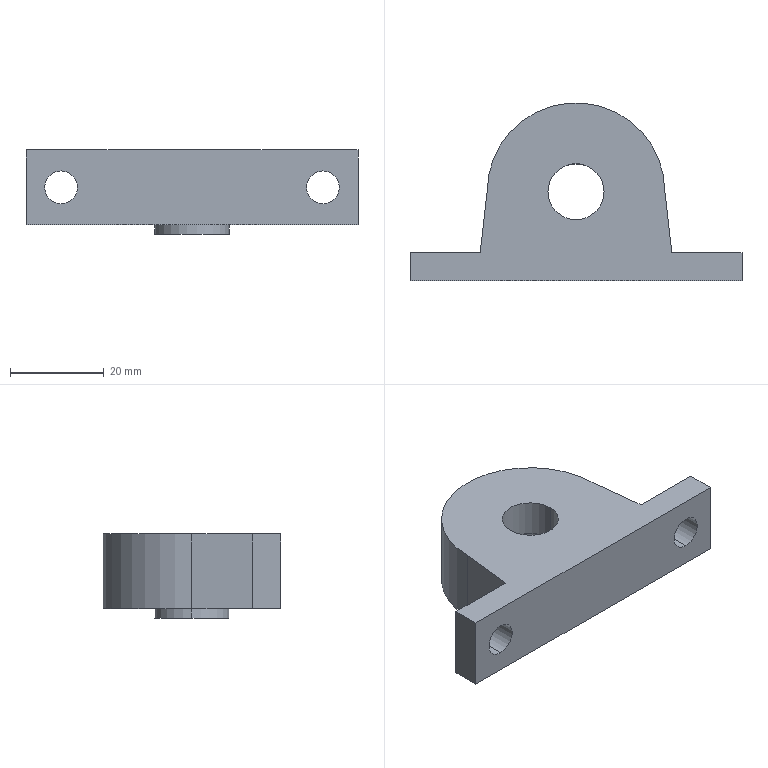Part | 2 solids | 22 faces | box 71 x 38 x 18 mm | volume 22713 mm3 | cylinder 11 | plane 11 | commonest cylinder face diameters 7 x4 12 x4 16 x2 38 x1
STEP:
#1=CARTESIAN_POINT('',(28.,-19.,4.5));
#2=VERTEX_POINT('',#1);
#3=CARTESIAN_POINT('',(28.,-19.,11.5));
#4=VERTEX_POINT('',#3);
#5=CARTESIAN_POINT('',(28.,-19.,8.));
#6=DIRECTION('',(0.,1.,0.));
#7=DIRECTION('',(-1.,0.,0.));
#8=AXIS2_PLACEMENT_3D('',#5,#6,#7);
#9=CIRCLE('',#8,3.5);
#10=EDGE_CURVE('',#2,#4,#9,.T.);
#11=ORIENTED_EDGE('',*,*,#10,.F.);
#12=CARTESIAN_POINT('',(28.,-13.,4.5));
#13=VERTEX_POINT('',#12);
#14=CARTESIAN_POINT('',(28.,-23.,4.5));
#15=DIRECTION('',(0.,1.,0.));
#16=VECTOR('',#15,1000.);
#17=LINE('',#14,#16);
#18=EDGE_CURVE('',#2,#13,#17,.T.);
#19=ORIENTED_EDGE('',*,*,#18,.T.);
#20=CARTESIAN_POINT('',(28.,-13.,11.5));
#21=VERTEX_POINT('',#20);
#22=CARTESIAN_POINT('',(28.,-13.,8.));
#23=DIRECTION('',(0.,1.,0.));
#24=DIRECTION('',(0.,0.,1.));
#25=AXIS2_PLACEMENT_3D('',#22,#23,#24);
#26=CIRCLE('',#25,3.5);
#27=EDGE_CURVE('',#13,#21,#26,.T.);
#28=ORIENTED_EDGE('',*,*,#27,.T.);
#29=CARTESIAN_POINT('',(28.,-23.,11.5));
#30=DIRECTION('',(0.,1.,0.));
#31=VECTOR('',#30,1000.);
#32=LINE('',#29,#31);
#33=EDGE_CURVE('',#4,#21,#32,.T.);
#34=ORIENTED_EDGE('',*,*,#33,.F.);
#35=EDGE_LOOP('',(#11,#19,#28,#34));
#36=FACE_OUTER_BOUND('',#35,.T.);
#37=CARTESIAN_POINT('',(28.,-23.,8.));
#38=DIRECTION('',(0.,1.,0.));
#39=DIRECTION('',(0.,0.,1.));
#40=AXIS2_PLACEMENT_3D('',#37,#38,#39);
#41=CYLINDRICAL_SURFACE('',#40,3.5);
#42=ADVANCED_FACE('',(#36),#41,.F.);
#43=CARTESIAN_POINT('',(-28.,-19.,4.5));
#44=VERTEX_POINT('',#43);
#45=CARTESIAN_POINT('',(-28.,-19.,11.5));
#46=VERTEX_POINT('',#45);
#47=CARTESIAN_POINT('',(-28.,-19.,8.));
#48=DIRECTION('',(0.,1.,0.));
#49=DIRECTION('',(-1.,0.,0.));
#50=AXIS2_PLACEMENT_3D('',#47,#48,#49);
#51=CIRCLE('',#50,3.5);
#52=EDGE_CURVE('',#44,#46,#51,.T.);
#53=ORIENTED_EDGE('',*,*,#52,.F.);
#54=CARTESIAN_POINT('',(-28.,-13.,4.5));
#55=VERTEX_POINT('',#54);
#56=CARTESIAN_POINT('',(-28.,-23.,4.5));
#57=DIRECTION('',(0.,1.,0.));
#58=VECTOR('',#57,1000.);
#59=LINE('',#56,#58);
#60=EDGE_CURVE('',#44,#55,#59,.T.);
#61=ORIENTED_EDGE('',*,*,#60,.T.);
#62=CARTESIAN_POINT('',(-28.,-13.,11.5));
#63=VERTEX_POINT('',#62);
#64=CARTESIAN_POINT('',(-28.,-13.,8.));
#65=DIRECTION('',(0.,1.,0.));
#66=DIRECTION('',(0.,0.,1.));
#67=AXIS2_PLACEMENT_3D('',#64,#65,#66);
#68=CIRCLE('',#67,3.5);
#69=EDGE_CURVE('',#55,#63,#68,.T.);
#70=ORIENTED_EDGE('',*,*,#69,.T.);
#71=CARTESIAN_POINT('',(-28.,-23.,11.5));
#72=DIRECTION('',(0.,1.,0.));
#73=VECTOR('',#72,1000.);
#74=LINE('',#71,#73);
#75=EDGE_CURVE('',#46,#63,#74,.T.);
#76=ORIENTED_EDGE('',*,*,#75,.F.);
#77=EDGE_LOOP('',(#53,#61,#70,#76));
#78=FACE_OUTER_BOUND('',#77,.T.);
#79=CARTESIAN_POINT('',(-28.,-23.,8.));
#80=DIRECTION('',(0.,1.,0.));
#81=DIRECTION('',(0.,0.,1.));
#82=AXIS2_PLACEMENT_3D('',#79,#80,#81);
#83=CYLINDRICAL_SURFACE('',#82,3.5);
#84=ADVANCED_FACE('',(#78),#83,.F.);
#85=CARTESIAN_POINT('',(-6.,0.,16.));
#86=VERTEX_POINT('',#85);
#87=CARTESIAN_POINT('',(6.,0.,16.));
#88=VERTEX_POINT('',#87);
#89=CARTESIAN_POINT('',(0.,0.,16.));
#90=DIRECTION('',(0.,0.,1.));
#91=DIRECTION('',(1.,0.,0.));
#92=AXIS2_PLACEMENT_3D('',#89,#90,#91);
#93=CIRCLE('',#92,6.);
#94=EDGE_CURVE('',#86,#88,#93,.T.);
#95=ORIENTED_EDGE('',*,*,#94,.T.);
#96=CARTESIAN_POINT('',(6.,0.,0.));
#97=VERTEX_POINT('',#96);
#98=CARTESIAN_POINT('',(6.,0.,16.));
#99=DIRECTION('',(0.,0.,-1.));
#100=VECTOR('',#99,1000.);
#101=LINE('',#98,#100);
#102=EDGE_CURVE('',#88,#97,#101,.T.);
#103=ORIENTED_EDGE('',*,*,#102,.T.);
#104=CARTESIAN_POINT('',(-6.,0.,0.));
#105=VERTEX_POINT('',#104);
#106=CARTESIAN_POINT('',(0.,0.,0.));
#107=DIRECTION('',(0.,0.,1.));
#108=DIRECTION('',(1.,0.,0.));
#109=AXIS2_PLACEMENT_3D('',#106,#107,#108);
#110=CIRCLE('',#109,6.);
#111=EDGE_CURVE('',#105,#97,#110,.T.);
#112=ORIENTED_EDGE('',*,*,#111,.F.);
#113=CARTESIAN_POINT('',(-6.,0.,16.));
#114=DIRECTION('',(0.,0.,-1.));
#115=VECTOR('',#114,1000.);
#116=LINE('',#113,#115);
#117=EDGE_CURVE('',#86,#105,#116,.T.);
#118=ORIENTED_EDGE('',*,*,#117,.F.);
#119=EDGE_LOOP('',(#95,#103,#112,#118));
#120=FACE_OUTER_BOUND('',#119,.T.);
#121=CARTESIAN_POINT('',(0.,0.,16.));
#122=DIRECTION('',(0.,0.,-1.));
#123=DIRECTION('',(-1.,0.,0.));
#124=AXIS2_PLACEMENT_3D('',#121,#122,#123);
#125=CYLINDRICAL_SURFACE('',#124,6.);
#126=ADVANCED_FACE('',(#120),#125,.F.);
#127=CARTESIAN_POINT('',(35.5,-13.,16.));
#128=VERTEX_POINT('',#127);
#129=CARTESIAN_POINT('',(20.5,-13.,16.));
#130=VERTEX_POINT('',#129);
#131=CARTESIAN_POINT('',(35.5,-13.,16.));
#132=DIRECTION('',(-1.,0.,0.));
#133=VECTOR('',#132,1000.);
#134=LINE('',#131,#133);
#135=EDGE_CURVE('',#128,#130,#134,.T.);
#136=ORIENTED_EDGE('',*,*,#135,.T.);
#137=CARTESIAN_POINT('',(19.,0.,16.));
#138=VERTEX_POINT('',#137);
#139=CARTESIAN_POINT('',(20.5,-13.,16.));
#140=DIRECTION('',(-0.1146,0.9934,0.));
#141=VECTOR('',#140,1000.);
#142=LINE('',#139,#141);
#143=EDGE_CURVE('',#130,#138,#142,.T.);
#144=ORIENTED_EDGE('',*,*,#143,.T.);
#145=CARTESIAN_POINT('',(-19.,0.,16.));
#146=VERTEX_POINT('',#145);
#147=CARTESIAN_POINT('',(0.,0.,16.));
#148=DIRECTION('',(0.,0.,1.));
#149=DIRECTION('',(1.,0.,0.));
#150=AXIS2_PLACEMENT_3D('',#147,#148,#149);
#151=CIRCLE('',#150,19.);
#152=EDGE_CURVE('',#138,#146,#151,.T.);
#153=ORIENTED_EDGE('',*,*,#152,.T.);
#154=CARTESIAN_POINT('',(-20.5,-13.,16.));
#155=VERTEX_POINT('',#154);
#156=CARTESIAN_POINT('',(-20.5,-13.,16.));
#157=DIRECTION('',(-0.1146,-0.9934,0.));
#158=VECTOR('',#157,1000.);
#159=LINE('',#156,#158);
#160=EDGE_CURVE('',#146,#155,#159,.T.);
#161=ORIENTED_EDGE('',*,*,#160,.T.);
#162=CARTESIAN_POINT('',(-35.5,-13.,16.));
#163=VERTEX_POINT('',#162);
#164=CARTESIAN_POINT('',(-35.5,-13.,16.));
#165=DIRECTION('',(-1.,0.,0.));
#166=VECTOR('',#165,1000.);
#167=LINE('',#164,#166);
#168=EDGE_CURVE('',#155,#163,#167,.T.);
#169=ORIENTED_EDGE('',*,*,#168,.T.);
#170=CARTESIAN_POINT('',(-35.5,-19.,16.));
#171=VERTEX_POINT('',#170);
#172=CARTESIAN_POINT('',(-35.5,-13.,16.));
#173=DIRECTION('',(0.,-1.,0.));
#174=VECTOR('',#173,1000.);
#175=LINE('',#172,#174);
#176=EDGE_CURVE('',#163,#171,#175,.T.);
#177=ORIENTED_EDGE('',*,*,#176,.T.);
#178=CARTESIAN_POINT('',(35.5,-19.,16.));
#179=VERTEX_POINT('',#178);
#180=CARTESIAN_POINT('',(-35.5,-19.,16.));
#181=DIRECTION('',(1.,0.,0.));
#182=VECTOR('',#181,1000.);
#183=LINE('',#180,#182);
#184=EDGE_CURVE('',#171,#179,#183,.T.);
#185=ORIENTED_EDGE('',*,*,#184,.T.);
#186=CARTESIAN_POINT('',(35.5,-19.,16.));
#187=DIRECTION('',(0.,1.,0.));
#188=VECTOR('',#187,1000.);
#189=LINE('',#186,#188);
#190=EDGE_CURVE('',#179,#128,#189,.T.);
#191=ORIENTED_EDGE('',*,*,#190,.T.);
#192=EDGE_LOOP('',(#136,#144,#153,#161,#169,#177,#185,#191));
#193=FACE_OUTER_BOUND('',#192,.T.);
#194=ORIENTED_EDGE('',*,*,#94,.F.);
#195=CARTESIAN_POINT('',(0.,0.,16.));
#196=DIRECTION('',(0.,0.,1.));
#197=DIRECTION('',(1.,0.,0.));
#198=AXIS2_PLACEMENT_3D('',#195,#196,#197);
#199=CIRCLE('',#198,6.);
#200=EDGE_CURVE('',#88,#86,#199,.T.);
#201=ORIENTED_EDGE('',*,*,#200,.F.);
#202=EDGE_LOOP('',(#194,#201));
#203=FACE_BOUND('',#202,.T.);
#204=CARTESIAN_POINT('',(0.,0.,16.));
#205=DIRECTION('',(0.,0.,1.));
#206=DIRECTION('',(1.,0.,0.));
#207=AXIS2_PLACEMENT_3D('',#204,#205,#206);
#208=PLANE('',#207);
#209=ADVANCED_FACE('',(#193,#203),#208,.T.);
#210=CARTESIAN_POINT('',(35.5,-13.,0.));
#211=VERTEX_POINT('',#210);
#212=CARTESIAN_POINT('',(20.5,-13.,0.));
#213=VERTEX_POINT('',#212);
#214=CARTESIAN_POINT('',(35.5,-13.,0.));
#215=DIRECTION('',(-1.,0.,0.));
#216=VECTOR('',#215,1000.);
#217=LINE('',#214,#216);
#218=EDGE_CURVE('',#211,#213,#217,.T.);
#219=ORIENTED_EDGE('',*,*,#218,.F.);
#220=CARTESIAN_POINT('',(35.5,-19.,0.));
#221=VERTEX_POINT('',#220);
#222=CARTESIAN_POINT('',(35.5,-19.,0.));
#223=DIRECTION('',(0.,1.,0.));
#224=VECTOR('',#223,1000.);
#225=LINE('',#222,#224);
#226=EDGE_CURVE('',#221,#211,#225,.T.);
#227=ORIENTED_EDGE('',*,*,#226,.F.);
#228=CARTESIAN_POINT('',(-35.5,-19.,0.));
#229=VERTEX_POINT('',#228);
#230=CARTESIAN_POINT('',(-35.5,-19.,0.));
#231=DIRECTION('',(1.,0.,0.));
#232=VECTOR('',#231,1000.);
#233=LINE('',#230,#232);
#234=EDGE_CURVE('',#229,#221,#233,.T.);
#235=ORIENTED_EDGE('',*,*,#234,.F.);
#236=CARTESIAN_POINT('',(-35.5,-13.,0.));
#237=VERTEX_POINT('',#236);
#238=CARTESIAN_POINT('',(-35.5,-13.,0.));
#239=DIRECTION('',(0.,-1.,0.));
#240=VECTOR('',#239,1000.);
#241=LINE('',#238,#240);
#242=EDGE_CURVE('',#237,#229,#241,.T.);
#243=ORIENTED_EDGE('',*,*,#242,.F.);
#244=CARTESIAN_POINT('',(-20.5,-13.,0.));
#245=VERTEX_POINT('',#244);
#246=CARTESIAN_POINT('',(-35.5,-13.,0.));
#247=DIRECTION('',(-1.,0.,0.));
#248=VECTOR('',#247,1000.);
#249=LINE('',#246,#248);
#250=EDGE_CURVE('',#245,#237,#249,.T.);
#251=ORIENTED_EDGE('',*,*,#250,.F.);
#252=CARTESIAN_POINT('',(-19.,0.,0.));
#253=VERTEX_POINT('',#252);
#254=CARTESIAN_POINT('',(-20.5,-13.,0.));
#255=DIRECTION('',(-0.1146,-0.9934,0.));
#256=VECTOR('',#255,1000.);
#257=LINE('',#254,#256);
#258=EDGE_CURVE('',#253,#245,#257,.T.);
#259=ORIENTED_EDGE('',*,*,#258,.F.);
#260=CARTESIAN_POINT('',(19.,0.,0.));
#261=VERTEX_POINT('',#260);
#262=CARTESIAN_POINT('',(0.,0.,0.));
#263=DIRECTION('',(0.,0.,1.));
#264=DIRECTION('',(1.,0.,0.));
#265=AXIS2_PLACEMENT_3D('',#262,#263,#264);
#266=CIRCLE('',#265,19.);
#267=EDGE_CURVE('',#261,#253,#266,.T.);
#268=ORIENTED_EDGE('',*,*,#267,.F.);
#269=CARTESIAN_POINT('',(20.5,-13.,0.));
#270=DIRECTION('',(-0.1146,0.9934,0.));
#271=VECTOR('',#270,1000.);
#272=LINE('',#269,#271);
#273=EDGE_CURVE('',#213,#261,#272,.T.);
#274=ORIENTED_EDGE('',*,*,#273,.F.);
#275=EDGE_LOOP('',(#219,#227,#235,#243,#251,#259,#268,#274));
#276=FACE_OUTER_BOUND('',#275,.T.);
#277=ORIENTED_EDGE('',*,*,#111,.T.);
#278=CARTESIAN_POINT('',(0.,0.,0.));
#279=DIRECTION('',(0.,0.,1.));
#280=DIRECTION('',(1.,0.,0.));
#281=AXIS2_PLACEMENT_3D('',#278,#279,#280);
#282=CIRCLE('',#281,6.);
#283=EDGE_CURVE('',#97,#105,#282,.T.);
#284=ORIENTED_EDGE('',*,*,#283,.T.);
#285=EDGE_LOOP('',(#277,#284));
#286=FACE_BOUND('',#285,.T.);
#287=CARTESIAN_POINT('',(0.,0.,0.));
#288=DIRECTION('',(0.,0.,1.));
#289=DIRECTION('',(1.,0.,0.));
#290=AXIS2_PLACEMENT_3D('',#287,#288,#289);
#291=PLANE('',#290);
#292=ADVANCED_FACE('',(#276,#286),#291,.F.);
#293=CARTESIAN_POINT('',(28.,-13.,8.));
#294=DIRECTION('',(0.,1.,0.));
#295=DIRECTION('',(0.,0.,1.));
#296=AXIS2_PLACEMENT_3D('',#293,#294,#295);
#297=CIRCLE('',#296,3.5);
#298=EDGE_CURVE('',#21,#13,#297,.T.);
#299=ORIENTED_EDGE('',*,*,#298,.F.);
#300=ORIENTED_EDGE('',*,*,#27,.F.);
#301=EDGE_LOOP('',(#299,#300));
#302=FACE_BOUND('',#301,.T.);
#303=ORIENTED_EDGE('',*,*,#218,.T.);
#304=CARTESIAN_POINT('',(20.5,-13.,16.));
#305=DIRECTION('',(0.,0.,-1.));
#306=VECTOR('',#305,1000.);
#307=LINE('',#304,#306);
#308=EDGE_CURVE('',#130,#213,#307,.T.);
#309=ORIENTED_EDGE('',*,*,#308,.F.);
#310=ORIENTED_EDGE('',*,*,#135,.F.);
#311=CARTESIAN_POINT('',(35.5,-13.,16.));
#312=DIRECTION('',(0.,0.,-1.));
#313=VECTOR('',#312,1000.);
#314=LINE('',#311,#313);
#315=EDGE_CURVE('',#128,#211,#314,.T.);
#316=ORIENTED_EDGE('',*,*,#315,.T.);
#317=EDGE_LOOP('',(#303,#309,#310,#316));
#318=FACE_OUTER_BOUND('',#317,.T.);
#319=CARTESIAN_POINT('',(35.5,-13.,16.));
#320=DIRECTION('',(0.,-1.,0.));
#321=DIRECTION('',(1.,0.,0.));
#322=AXIS2_PLACEMENT_3D('',#319,#320,#321);
#323=PLANE('',#322);
#324=ADVANCED_FACE('',(#302,#318),#323,.F.);
#325=ORIENTED_EDGE('',*,*,#273,.T.);
#326=CARTESIAN_POINT('',(19.,0.,16.));
#327=DIRECTION('',(0.,0.,-1.));
#328=VECTOR('',#327,1000.);
#329=LINE('',#326,#328);
#330=EDGE_CURVE('',#138,#261,#329,.T.);
#331=ORIENTED_EDGE('',*,*,#330,.F.);
#332=ORIENTED_EDGE('',*,*,#143,.F.);
#333=ORIENTED_EDGE('',*,*,#308,.T.);
#334=EDGE_LOOP('',(#325,#331,#332,#333));
#335=FACE_OUTER_BOUND('',#334,.T.);
#336=CARTESIAN_POINT('',(20.5,-13.,16.));
#337=DIRECTION('',(-0.9934,-0.1146,0.));
#338=DIRECTION('',(0.1146,-0.9934,0.));
#339=AXIS2_PLACEMENT_3D('',#336,#337,#338);
#340=PLANE('',#339);
#341=ADVANCED_FACE('',(#335),#340,.F.);
#342=ORIENTED_EDGE('',*,*,#267,.T.);
#343=CARTESIAN_POINT('',(-19.,0.,16.));
#344=DIRECTION('',(0.,0.,-1.));
#345=VECTOR('',#344,1000.);
#346=LINE('',#343,#345);
#347=EDGE_CURVE('',#146,#253,#346,.T.);
#348=ORIENTED_EDGE('',*,*,#347,.F.);
#349=ORIENTED_EDGE('',*,*,#152,.F.);
#350=ORIENTED_EDGE('',*,*,#330,.T.);
#351=EDGE_LOOP('',(#342,#348,#349,#350));
#352=FACE_OUTER_BOUND('',#351,.T.);
#353=CARTESIAN_POINT('',(0.,0.,16.));
#354=DIRECTION('',(0.,0.,-1.));
#355=DIRECTION('',(-1.,0.,0.));
#356=AXIS2_PLACEMENT_3D('',#353,#354,#355);
#357=CYLINDRICAL_SURFACE('',#356,19.);
#358=ADVANCED_FACE('',(#352),#357,.T.);
#359=ORIENTED_EDGE('',*,*,#258,.T.);
#360=CARTESIAN_POINT('',(-20.5,-13.,16.));
#361=DIRECTION('',(0.,0.,-1.));
#362=VECTOR('',#361,1000.);
#363=LINE('',#360,#362);
#364=EDGE_CURVE('',#155,#245,#363,.T.);
#365=ORIENTED_EDGE('',*,*,#364,.F.);
#366=ORIENTED_EDGE('',*,*,#160,.F.);
#367=ORIENTED_EDGE('',*,*,#347,.T.);
#368=EDGE_LOOP('',(#359,#365,#366,#367));
#369=FACE_OUTER_BOUND('',#368,.T.);
#370=CARTESIAN_POINT('',(-20.5,-13.,16.));
#371=DIRECTION('',(0.9934,-0.1146,0.));
#372=DIRECTION('',(0.1146,0.9934,0.));
#373=AXIS2_PLACEMENT_3D('',#370,#371,#372);
#374=PLANE('',#373);
#375=ADVANCED_FACE('',(#369),#374,.F.);
#376=CARTESIAN_POINT('',(-28.,-13.,8.));
#377=DIRECTION('',(0.,1.,0.));
#378=DIRECTION('',(0.,0.,1.));
#379=AXIS2_PLACEMENT_3D('',#376,#377,#378);
#380=CIRCLE('',#379,3.5);
#381=EDGE_CURVE('',#63,#55,#380,.T.);
#382=ORIENTED_EDGE('',*,*,#381,.F.);
#383=ORIENTED_EDGE('',*,*,#69,.F.);
#384=EDGE_LOOP('',(#382,#383));
#385=FACE_BOUND('',#384,.T.);
#386=ORIENTED_EDGE('',*,*,#250,.T.);
#387=CARTESIAN_POINT('',(-35.5,-13.,16.));
#388=DIRECTION('',(0.,0.,-1.));
#389=VECTOR('',#388,1000.);
#390=LINE('',#387,#389);
#391=EDGE_CURVE('',#163,#237,#390,.T.);
#392=ORIENTED_EDGE('',*,*,#391,.F.);
#393=ORIENTED_EDGE('',*,*,#168,.F.);
#394=ORIENTED_EDGE('',*,*,#364,.T.);
#395=EDGE_LOOP('',(#386,#392,#393,#394));
#396=FACE_OUTER_BOUND('',#395,.T.);
#397=CARTESIAN_POINT('',(-35.5,-13.,16.));
#398=DIRECTION('',(0.,-1.,0.));
#399=DIRECTION('',(0.,0.,-1.));
#400=AXIS2_PLACEMENT_3D('',#397,#398,#399);
#401=PLANE('',#400);
#402=ADVANCED_FACE('',(#385,#396),#401,.F.);
#403=ORIENTED_EDGE('',*,*,#242,.T.);
#404=CARTESIAN_POINT('',(-35.5,-19.,16.));
#405=DIRECTION('',(0.,0.,-1.));
#406=VECTOR('',#405,1000.);
#407=LINE('',#404,#406);
#408=EDGE_CURVE('',#171,#229,#407,.T.);
#409=ORIENTED_EDGE('',*,*,#408,.F.);
#410=ORIENTED_EDGE('',*,*,#176,.F.);
#411=ORIENTED_EDGE('',*,*,#391,.T.);
#412=EDGE_LOOP('',(#403,#409,#410,#411));
#413=FACE_OUTER_BOUND('',#412,.T.);
#414=CARTESIAN_POINT('',(-35.5,-13.,16.));
#415=DIRECTION('',(1.,0.,0.));
#416=DIRECTION('',(0.,0.,-1.));
#417=AXIS2_PLACEMENT_3D('',#414,#415,#416);
#418=PLANE('',#417);
#419=ADVANCED_FACE('',(#413),#418,.F.);
#420=CARTESIAN_POINT('',(28.,-19.,8.));
#421=DIRECTION('',(0.,1.,0.));
#422=DIRECTION('',(-1.,0.,0.));
#423=AXIS2_PLACEMENT_3D('',#420,#421,#422);
#424=CIRCLE('',#423,3.5);
#425=EDGE_CURVE('',#4,#2,#424,.T.);
#426=ORIENTED_EDGE('',*,*,#425,.T.);
#427=ORIENTED_EDGE('',*,*,#10,.T.);
#428=EDGE_LOOP('',(#426,#427));
#429=FACE_BOUND('',#428,.T.);
#430=CARTESIAN_POINT('',(-28.,-19.,8.));
#431=DIRECTION('',(0.,1.,0.));
#432=DIRECTION('',(-1.,0.,0.));
#433=AXIS2_PLACEMENT_3D('',#430,#431,#432);
#434=CIRCLE('',#433,3.5);
#435=EDGE_CURVE('',#46,#44,#434,.T.);
#436=ORIENTED_EDGE('',*,*,#435,.T.);
#437=ORIENTED_EDGE('',*,*,#52,.T.);
#438=EDGE_LOOP('',(#436,#437));
#439=FACE_BOUND('',#438,.T.);
#440=ORIENTED_EDGE('',*,*,#234,.T.);
#441=CARTESIAN_POINT('',(35.5,-19.,16.));
#442=DIRECTION('',(0.,0.,-1.));
#443=VECTOR('',#442,1000.);
#444=LINE('',#441,#443);
#445=EDGE_CURVE('',#179,#221,#444,.T.);
#446=ORIENTED_EDGE('',*,*,#445,.F.);
#447=ORIENTED_EDGE('',*,*,#184,.F.);
#448=ORIENTED_EDGE('',*,*,#408,.T.);
#449=EDGE_LOOP('',(#440,#446,#447,#448));
#450=FACE_OUTER_BOUND('',#449,.T.);
#451=CARTESIAN_POINT('',(-35.5,-19.,16.));
#452=DIRECTION('',(0.,1.,0.));
#453=DIRECTION('',(-1.,0.,0.));
#454=AXIS2_PLACEMENT_3D('',#451,#452,#453);
#455=PLANE('',#454);
#456=ADVANCED_FACE('',(#429,#439,#450),#455,.F.);
#457=ORIENTED_EDGE('',*,*,#226,.T.);
#458=ORIENTED_EDGE('',*,*,#315,.F.);
#459=ORIENTED_EDGE('',*,*,#190,.F.);
#460=ORIENTED_EDGE('',*,*,#445,.T.);
#461=EDGE_LOOP('',(#457,#458,#459,#460));
#462=FACE_OUTER_BOUND('',#461,.T.);
#463=CARTESIAN_POINT('',(35.5,-19.,16.));
#464=DIRECTION('',(-1.,0.,0.));
#465=DIRECTION('',(0.,0.,1.));
#466=AXIS2_PLACEMENT_3D('',#463,#464,#465);
#467=PLANE('',#466);
#468=ADVANCED_FACE('',(#462),#467,.F.);
#469=ORIENTED_EDGE('',*,*,#102,.F.);
#470=ORIENTED_EDGE('',*,*,#200,.T.);
#471=ORIENTED_EDGE('',*,*,#117,.T.);
#472=ORIENTED_EDGE('',*,*,#283,.F.);
#473=EDGE_LOOP('',(#469,#470,#471,#472));
#474=FACE_OUTER_BOUND('',#473,.T.);
#475=CARTESIAN_POINT('',(0.,0.,16.));
#476=DIRECTION('',(0.,0.,-1.));
#477=DIRECTION('',(-1.,0.,0.));
#478=AXIS2_PLACEMENT_3D('',#475,#476,#477);
#479=CYLINDRICAL_SURFACE('',#478,6.);
#480=ADVANCED_FACE('',(#474),#479,.F.);
#481=ORIENTED_EDGE('',*,*,#60,.F.);
#482=ORIENTED_EDGE('',*,*,#435,.F.);
#483=ORIENTED_EDGE('',*,*,#75,.T.);
#484=ORIENTED_EDGE('',*,*,#381,.T.);
#485=EDGE_LOOP('',(#481,#482,#483,#484));
#486=FACE_OUTER_BOUND('',#485,.T.);
#487=CARTESIAN_POINT('',(-28.,-23.,8.));
#488=DIRECTION('',(0.,1.,0.));
#489=DIRECTION('',(0.,0.,1.));
#490=AXIS2_PLACEMENT_3D('',#487,#488,#489);
#491=CYLINDRICAL_SURFACE('',#490,3.5);
#492=ADVANCED_FACE('',(#486),#491,.F.);
#493=ORIENTED_EDGE('',*,*,#18,.F.);
#494=ORIENTED_EDGE('',*,*,#425,.F.);
#495=ORIENTED_EDGE('',*,*,#33,.T.);
#496=ORIENTED_EDGE('',*,*,#298,.T.);
#497=EDGE_LOOP('',(#493,#494,#495,#496));
#498=FACE_OUTER_BOUND('',#497,.T.);
#499=CARTESIAN_POINT('',(28.,-23.,8.));
#500=DIRECTION('',(0.,1.,0.));
#501=DIRECTION('',(0.,0.,1.));
#502=AXIS2_PLACEMENT_3D('',#499,#500,#501);
#503=CYLINDRICAL_SURFACE('',#502,3.5);
#504=ADVANCED_FACE('',(#498),#503,.F.);
#505=CLOSED_SHELL('',(#42,#84,#126,#209,#292,#324,#341,#358,#375,#402,#419,#456,#468,#480,#492,#504));
#506=MANIFOLD_SOLID_BREP('',#505);
#507=CARTESIAN_POINT('',(6.,0.,-2.));
#508=VERTEX_POINT('',#507);
#509=CARTESIAN_POINT('',(-6.,0.,-2.));
#510=VERTEX_POINT('',#509);
#511=CARTESIAN_POINT('',(0.,0.,-2.));
#512=DIRECTION('',(0.,0.,-1.));
#513=DIRECTION('',(-1.,0.,0.));
#514=AXIS2_PLACEMENT_3D('',#511,#512,#513);
#515=CIRCLE('',#514,6.);
#516=EDGE_CURVE('',#508,#510,#515,.T.);
#517=ORIENTED_EDGE('',*,*,#516,.T.);
#518=CARTESIAN_POINT('',(-6.,0.,8.));
#519=VERTEX_POINT('',#518);
#520=CARTESIAN_POINT('',(-6.,0.,-2.));
#521=DIRECTION('',(0.,0.,1.));
#522=VECTOR('',#521,1000.);
#523=LINE('',#520,#522);
#524=EDGE_CURVE('',#510,#519,#523,.T.);
#525=ORIENTED_EDGE('',*,*,#524,.T.);
#526=CARTESIAN_POINT('',(6.,0.,8.));
#527=VERTEX_POINT('',#526);
#528=CARTESIAN_POINT('',(0.,0.,8.));
#529=DIRECTION('',(0.,0.,-1.));
#530=DIRECTION('',(-1.,0.,0.));
#531=AXIS2_PLACEMENT_3D('',#528,#529,#530);
#532=CIRCLE('',#531,6.);
#533=EDGE_CURVE('',#527,#519,#532,.T.);
#534=ORIENTED_EDGE('',*,*,#533,.F.);
#535=CARTESIAN_POINT('',(6.,0.,-2.));
#536=DIRECTION('',(0.,0.,1.));
#537=VECTOR('',#536,1000.);
#538=LINE('',#535,#537);
#539=EDGE_CURVE('',#508,#527,#538,.T.);
#540=ORIENTED_EDGE('',*,*,#539,.F.);
#541=EDGE_LOOP('',(#517,#525,#534,#540));
#542=FACE_OUTER_BOUND('',#541,.T.);
#543=CARTESIAN_POINT('',(0.,0.,-2.));
#544=DIRECTION('',(0.,0.,1.));
#545=DIRECTION('',(1.,0.,0.));
#546=AXIS2_PLACEMENT_3D('',#543,#544,#545);
#547=CYLINDRICAL_SURFACE('',#546,6.);
#548=ADVANCED_FACE('',(#542),#547,.F.);
#549=CARTESIAN_POINT('',(-8.,0.,-2.));
#550=VERTEX_POINT('',#549);
#551=CARTESIAN_POINT('',(8.,0.,-2.));
#552=VERTEX_POINT('',#551);
#553=CARTESIAN_POINT('',(0.,0.,-2.));
#554=DIRECTION('',(0.,0.,-1.));
#555=DIRECTION('',(-1.,0.,0.));
#556=AXIS2_PLACEMENT_3D('',#553,#554,#555);
#557=CIRCLE('',#556,8.);
#558=EDGE_CURVE('',#550,#552,#557,.T.);
#559=ORIENTED_EDGE('',*,*,#558,.F.);
#560=CARTESIAN_POINT('',(-8.,0.,8.));
#561=VERTEX_POINT('',#560);
#562=CARTESIAN_POINT('',(-8.,0.,-2.));
#563=DIRECTION('',(0.,0.,1.));
#564=VECTOR('',#563,1000.);
#565=LINE('',#562,#564);
#566=EDGE_CURVE('',#550,#561,#565,.T.);
#567=ORIENTED_EDGE('',*,*,#566,.T.);
#568=CARTESIAN_POINT('',(8.,0.,8.));
#569=VERTEX_POINT('',#568);
#570=CARTESIAN_POINT('',(0.,0.,8.));
#571=DIRECTION('',(0.,0.,-1.));
#572=DIRECTION('',(-1.,0.,0.));
#573=AXIS2_PLACEMENT_3D('',#570,#571,#572);
#574=CIRCLE('',#573,8.);
#575=EDGE_CURVE('',#561,#569,#574,.T.);
#576=ORIENTED_EDGE('',*,*,#575,.T.);
#577=CARTESIAN_POINT('',(8.,0.,-2.));
#578=DIRECTION('',(0.,0.,1.));
#579=VECTOR('',#578,1000.);
#580=LINE('',#577,#579);
#581=EDGE_CURVE('',#552,#569,#580,.T.);
#582=ORIENTED_EDGE('',*,*,#581,.F.);
#583=EDGE_LOOP('',(#559,#567,#576,#582));
#584=FACE_OUTER_BOUND('',#583,.T.);
#585=CARTESIAN_POINT('',(0.,0.,-2.));
#586=DIRECTION('',(0.,0.,1.));
#587=DIRECTION('',(1.,0.,0.));
#588=AXIS2_PLACEMENT_3D('',#585,#586,#587);
#589=CYLINDRICAL_SURFACE('',#588,8.);
#590=ADVANCED_FACE('',(#584),#589,.T.);
#591=CARTESIAN_POINT('',(0.,0.,-2.));
#592=DIRECTION('',(0.,0.,-1.));
#593=DIRECTION('',(-1.,0.,0.));
#594=AXIS2_PLACEMENT_3D('',#591,#592,#593);
#595=CIRCLE('',#594,8.);
#596=EDGE_CURVE('',#552,#550,#595,.T.);
#597=ORIENTED_EDGE('',*,*,#596,.T.);
#598=ORIENTED_EDGE('',*,*,#558,.T.);
#599=EDGE_LOOP('',(#597,#598));
#600=FACE_OUTER_BOUND('',#599,.T.);
#601=ORIENTED_EDGE('',*,*,#516,.F.);
#602=CARTESIAN_POINT('',(0.,0.,-2.));
#603=DIRECTION('',(0.,0.,-1.));
#604=DIRECTION('',(-1.,0.,0.));
#605=AXIS2_PLACEMENT_3D('',#602,#603,#604);
#606=CIRCLE('',#605,6.);
#607=EDGE_CURVE('',#510,#508,#606,.T.);
#608=ORIENTED_EDGE('',*,*,#607,.F.);
#609=EDGE_LOOP('',(#601,#608));
#610=FACE_BOUND('',#609,.T.);
#611=CARTESIAN_POINT('',(0.,0.,-2.));
#612=DIRECTION('',(0.,0.,-1.));
#613=DIRECTION('',(-1.,0.,0.));
#614=AXIS2_PLACEMENT_3D('',#611,#612,#613);
#615=PLANE('',#614);
#616=ADVANCED_FACE('',(#600,#610),#615,.T.);
#617=CARTESIAN_POINT('',(0.,0.,8.));
#618=DIRECTION('',(0.,0.,-1.));
#619=DIRECTION('',(-1.,0.,0.));
#620=AXIS2_PLACEMENT_3D('',#617,#618,#619);
#621=CIRCLE('',#620,8.);
#622=EDGE_CURVE('',#569,#561,#621,.T.);
#623=ORIENTED_EDGE('',*,*,#622,.F.);
#624=ORIENTED_EDGE('',*,*,#575,.F.);
#625=EDGE_LOOP('',(#623,#624));
#626=FACE_OUTER_BOUND('',#625,.T.);
#627=ORIENTED_EDGE('',*,*,#533,.T.);
#628=CARTESIAN_POINT('',(0.,0.,8.));
#629=DIRECTION('',(0.,0.,-1.));
#630=DIRECTION('',(-1.,0.,0.));
#631=AXIS2_PLACEMENT_3D('',#628,#629,#630);
#632=CIRCLE('',#631,6.);
#633=EDGE_CURVE('',#519,#527,#632,.T.);
#634=ORIENTED_EDGE('',*,*,#633,.T.);
#635=EDGE_LOOP('',(#627,#634));
#636=FACE_BOUND('',#635,.T.);
#637=CARTESIAN_POINT('',(0.,0.,8.));
#638=DIRECTION('',(0.,0.,-1.));
#639=DIRECTION('',(-1.,0.,0.));
#640=AXIS2_PLACEMENT_3D('',#637,#638,#639);
#641=PLANE('',#640);
#642=ADVANCED_FACE('',(#626,#636),#641,.F.);
#643=ORIENTED_EDGE('',*,*,#566,.F.);
#644=ORIENTED_EDGE('',*,*,#596,.F.);
#645=ORIENTED_EDGE('',*,*,#581,.T.);
#646=ORIENTED_EDGE('',*,*,#622,.T.);
#647=EDGE_LOOP('',(#643,#644,#645,#646));
#648=FACE_OUTER_BOUND('',#647,.T.);
#649=CARTESIAN_POINT('',(0.,0.,-2.));
#650=DIRECTION('',(0.,0.,1.));
#651=DIRECTION('',(1.,0.,0.));
#652=AXIS2_PLACEMENT_3D('',#649,#650,#651);
#653=CYLINDRICAL_SURFACE('',#652,8.);
#654=ADVANCED_FACE('',(#648),#653,.T.);
#655=ORIENTED_EDGE('',*,*,#524,.F.);
#656=ORIENTED_EDGE('',*,*,#607,.T.);
#657=ORIENTED_EDGE('',*,*,#539,.T.);
#658=ORIENTED_EDGE('',*,*,#633,.F.);
#659=EDGE_LOOP('',(#655,#656,#657,#658));
#660=FACE_OUTER_BOUND('',#659,.T.);
#661=CARTESIAN_POINT('',(0.,0.,-2.));
#662=DIRECTION('',(0.,0.,1.));
#663=DIRECTION('',(1.,0.,0.));
#664=AXIS2_PLACEMENT_3D('',#661,#662,#663);
#665=CYLINDRICAL_SURFACE('',#664,6.);
#666=ADVANCED_FACE('',(#660),#665,.F.);
#667=CLOSED_SHELL('',(#548,#590,#616,#642,#654,#666));
#668=MANIFOLD_SOLID_BREP('',#667);
#669=CARTESIAN_POINT('',(0.,0.,0.));
#670=DIRECTION('',(0.,0.,1.));
#671=DIRECTION('',(1.,0.,0.));
#672=AXIS2_PLACEMENT_3D('',#669,#670,#671);
#673=(LENGTH_UNIT()NAMED_UNIT(*)SI_UNIT(.MILLI.,.METRE.));
#674=UNCERTAINTY_MEASURE_WITH_UNIT(LENGTH_MEASURE(0.00001),#673,'','');
#675=(NAMED_UNIT(*)PLANE_ANGLE_UNIT()SI_UNIT($,.RADIAN.));
#676=(NAMED_UNIT(*)SI_UNIT($,.STERADIAN.)SOLID_ANGLE_UNIT());
#677=(GEOMETRIC_REPRESENTATION_CONTEXT(3)GLOBAL_UNCERTAINTY_ASSIGNED_CONTEXT((#674))GLOBAL_UNIT_ASSIGNED_CONTEXT((#673,#675,#676))REPRESENTATION_CONTEXT('',''));
#678=ADVANCED_BREP_SHAPE_REPRESENTATION('',(#506,#668,#672),#677);